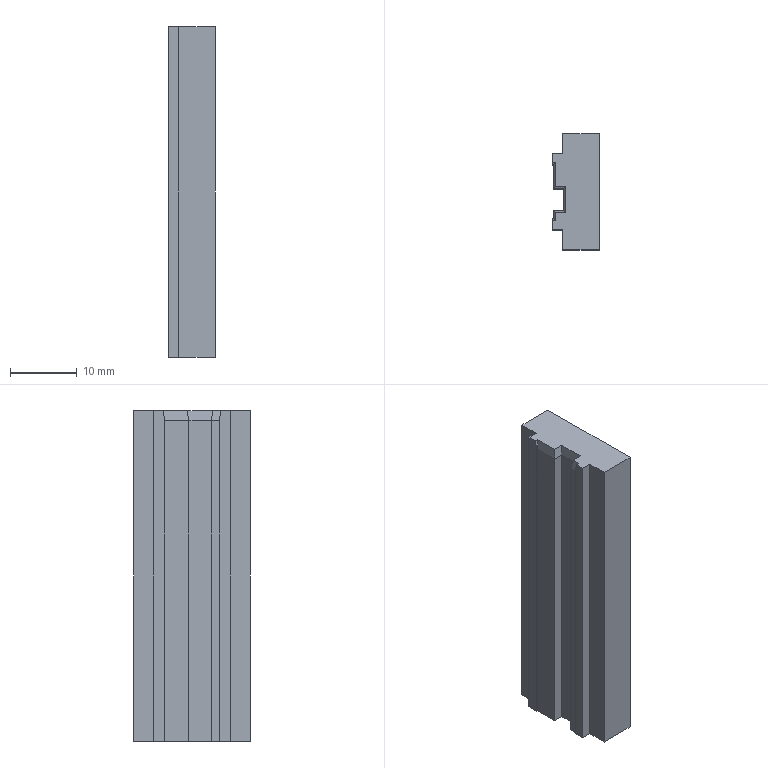Part | SolidWorks | features ICE 3, Chamfer 2, RefAxis 2, Extrusion 1, MirrorPattern 1, RevCut 1 | 1 solid | 33 faces | box 7 x 17.4 x 49.4 mm | volume 5230 mm3 | plane 25 | cone 4 | sphere 4
STEP:
#1=CARTESIAN_POINT('',(5.617,0.,19.076));
#2=VERTEX_POINT('',#1);
#3=CARTESIAN_POINT('',(5.617,0.,20.924));
#4=VERTEX_POINT('',#3);
#5=CARTESIAN_POINT('',(5.617,0.,20.));
#6=DIRECTION('',(1.,0.,0.));
#7=DIRECTION('',(0.,0.,-1.));
#8=AXIS2_PLACEMENT_3D('',#5,#6,#7);
#9=CIRCLE('',#8,0.9239);
#10=EDGE_CURVE('',#2,#4,#9,.T.);
#11=ORIENTED_EDGE('',*,*,#10,.F.);
#12=CARTESIAN_POINT('',(7.,0.,18.503));
#13=VERTEX_POINT('',#12);
#14=CARTESIAN_POINT('',(7.,0.,18.503));
#15=DIRECTION('',(0.9239,0.,-0.3827));
#16=VECTOR('',#15,1000.);
#17=LINE('',#14,#16);
#18=EDGE_CURVE('',#2,#13,#17,.T.);
#19=ORIENTED_EDGE('',*,*,#18,.T.);
#20=CARTESIAN_POINT('',(7.,0.,21.497));
#21=VERTEX_POINT('',#20);
#22=CARTESIAN_POINT('',(7.,0.,20.));
#23=DIRECTION('',(1.,0.,0.));
#24=DIRECTION('',(0.,0.,-1.));
#25=AXIS2_PLACEMENT_3D('',#22,#23,#24);
#26=CIRCLE('',#25,1.497);
#27=EDGE_CURVE('',#13,#21,#26,.T.);
#28=ORIENTED_EDGE('',*,*,#27,.T.);
#29=CARTESIAN_POINT('',(7.,0.,21.497));
#30=DIRECTION('',(0.9239,0.,0.3827));
#31=VECTOR('',#30,1000.);
#32=LINE('',#29,#31);
#33=EDGE_CURVE('',#4,#21,#32,.T.);
#34=ORIENTED_EDGE('',*,*,#33,.F.);
#35=EDGE_LOOP('',(#11,#19,#28,#34));
#36=FACE_OUTER_BOUND('',#35,.T.);
#37=CARTESIAN_POINT('',(7.,0.,20.));
#38=DIRECTION('',(1.,0.,0.));
#39=DIRECTION('',(0.,0.,1.));
#40=AXIS2_PLACEMENT_3D('',#37,#38,#39);
#41=CONICAL_SURFACE('',#40,1.497,0.3927);
#42=ADVANCED_FACE('',(#36),#41,.F.);
#43=CARTESIAN_POINT('',(5.617,0.,20.));
#44=DIRECTION('',(1.,0.,0.));
#45=DIRECTION('',(0.,0.,-1.));
#46=AXIS2_PLACEMENT_3D('',#43,#44,#45);
#47=CIRCLE('',#46,0.9239);
#48=EDGE_CURVE('',#4,#2,#47,.T.);
#49=ORIENTED_EDGE('',*,*,#48,.T.);
#50=CARTESIAN_POINT('',(5.,0.,20.));
#51=VERTEX_POINT('',#50);
#52=CARTESIAN_POINT('',(6.,0.,20.));
#53=DIRECTION('',(0.,1.,0.));
#54=DIRECTION('',(0.,0.,1.));
#55=AXIS2_PLACEMENT_3D('',#52,#53,#54);
#56=CIRCLE('',#55,1.);
#57=EDGE_CURVE('',#2,#51,#56,.T.);
#58=ORIENTED_EDGE('',*,*,#57,.T.);
#59=CARTESIAN_POINT('',(6.,0.,20.));
#60=DIRECTION('',(0.,-1.,0.));
#61=DIRECTION('',(0.,0.,-1.));
#62=AXIS2_PLACEMENT_3D('',#59,#60,#61);
#63=CIRCLE('',#62,1.);
#64=EDGE_CURVE('',#4,#51,#63,.T.);
#65=ORIENTED_EDGE('',*,*,#64,.F.);
#66=EDGE_LOOP('',(#49,#58,#65));
#67=FACE_OUTER_BOUND('',#66,.T.);
#68=CARTESIAN_POINT('',(6.,0.,20.));
#69=DIRECTION('',(0.,1.,0.));
#70=DIRECTION('',(0.,0.,1.));
#71=AXIS2_PLACEMENT_3D('',#68,#69,#70);
#72=SPHERICAL_SURFACE('',#71,1.);
#73=ADVANCED_FACE('',(#67),#72,.F.);
#74=CARTESIAN_POINT('',(5.617,0.,-20.924));
#75=VERTEX_POINT('',#74);
#76=CARTESIAN_POINT('',(5.617,0.,-19.076));
#77=VERTEX_POINT('',#76);
#78=CARTESIAN_POINT('',(5.617,0.,-20.));
#79=DIRECTION('',(-1.,0.,0.));
#80=DIRECTION('',(0.,0.,1.));
#81=AXIS2_PLACEMENT_3D('',#78,#79,#80);
#82=CIRCLE('',#81,0.9239);
#83=EDGE_CURVE('',#75,#77,#82,.T.);
#84=ORIENTED_EDGE('',*,*,#83,.T.);
#85=CARTESIAN_POINT('',(7.,0.,-18.503));
#86=VERTEX_POINT('',#85);
#87=CARTESIAN_POINT('',(7.,0.,-18.503));
#88=DIRECTION('',(0.9239,0.,0.3827));
#89=VECTOR('',#88,1000.);
#90=LINE('',#87,#89);
#91=EDGE_CURVE('',#77,#86,#90,.T.);
#92=ORIENTED_EDGE('',*,*,#91,.T.);
#93=CARTESIAN_POINT('',(7.,0.,-21.497));
#94=VERTEX_POINT('',#93);
#95=CARTESIAN_POINT('',(7.,0.,-20.));
#96=DIRECTION('',(-1.,0.,0.));
#97=DIRECTION('',(0.,0.,1.));
#98=AXIS2_PLACEMENT_3D('',#95,#96,#97);
#99=CIRCLE('',#98,1.497);
#100=EDGE_CURVE('',#94,#86,#99,.T.);
#101=ORIENTED_EDGE('',*,*,#100,.F.);
#102=CARTESIAN_POINT('',(7.,0.,-21.497));
#103=DIRECTION('',(0.9239,0.,-0.3827));
#104=VECTOR('',#103,1000.);
#105=LINE('',#102,#104);
#106=EDGE_CURVE('',#75,#94,#105,.T.);
#107=ORIENTED_EDGE('',*,*,#106,.F.);
#108=EDGE_LOOP('',(#84,#92,#101,#107));
#109=FACE_OUTER_BOUND('',#108,.T.);
#110=CARTESIAN_POINT('',(7.,0.,-20.));
#111=DIRECTION('',(1.,0.,0.));
#112=DIRECTION('',(0.,0.,-1.));
#113=AXIS2_PLACEMENT_3D('',#110,#111,#112);
#114=CONICAL_SURFACE('',#113,1.497,0.3927);
#115=ADVANCED_FACE('',(#109),#114,.F.);
#116=CARTESIAN_POINT('',(5.617,0.,-20.));
#117=DIRECTION('',(-1.,0.,0.));
#118=DIRECTION('',(0.,0.,1.));
#119=AXIS2_PLACEMENT_3D('',#116,#117,#118);
#120=CIRCLE('',#119,0.9239);
#121=EDGE_CURVE('',#77,#75,#120,.T.);
#122=ORIENTED_EDGE('',*,*,#121,.F.);
#123=CARTESIAN_POINT('',(5.,0.,-20.));
#124=VERTEX_POINT('',#123);
#125=CARTESIAN_POINT('',(6.,0.,-20.));
#126=DIRECTION('',(0.,-1.,0.));
#127=DIRECTION('',(0.,0.,-1.));
#128=AXIS2_PLACEMENT_3D('',#125,#126,#127);
#129=CIRCLE('',#128,1.);
#130=EDGE_CURVE('',#77,#124,#129,.T.);
#131=ORIENTED_EDGE('',*,*,#130,.T.);
#132=CARTESIAN_POINT('',(6.,0.,-20.));
#133=DIRECTION('',(0.,1.,0.));
#134=DIRECTION('',(0.,0.,1.));
#135=AXIS2_PLACEMENT_3D('',#132,#133,#134);
#136=CIRCLE('',#135,1.);
#137=EDGE_CURVE('',#75,#124,#136,.T.);
#138=ORIENTED_EDGE('',*,*,#137,.F.);
#139=EDGE_LOOP('',(#122,#131,#138));
#140=FACE_OUTER_BOUND('',#139,.T.);
#141=CARTESIAN_POINT('',(6.,0.,-20.));
#142=DIRECTION('',(0.,-1.,0.));
#143=DIRECTION('',(0.,0.,-1.));
#144=AXIS2_PLACEMENT_3D('',#141,#142,#143);
#145=SPHERICAL_SURFACE('',#144,1.);
#146=ADVANCED_FACE('',(#140),#145,.F.);
#147=CARTESIAN_POINT('',(1.5,8.7,24.7));
#148=VERTEX_POINT('',#147);
#149=CARTESIAN_POINT('',(1.5,8.7,-24.7));
#150=VERTEX_POINT('',#149);
#151=CARTESIAN_POINT('',(1.5,8.7,-24.7));
#152=DIRECTION('',(0.,0.,-1.));
#153=VECTOR('',#152,1000.);
#154=LINE('',#151,#153);
#155=EDGE_CURVE('',#148,#150,#154,.T.);
#156=ORIENTED_EDGE('',*,*,#155,.F.);
#157=CARTESIAN_POINT('',(7.,8.7,24.7));
#158=VERTEX_POINT('',#157);
#159=CARTESIAN_POINT('',(7.,8.7,24.7));
#160=DIRECTION('',(-1.,0.,0.));
#161=VECTOR('',#160,1000.);
#162=LINE('',#159,#161);
#163=EDGE_CURVE('',#158,#148,#162,.T.);
#164=ORIENTED_EDGE('',*,*,#163,.F.);
#165=CARTESIAN_POINT('',(7.,8.7,-24.7));
#166=VERTEX_POINT('',#165);
#167=CARTESIAN_POINT('',(7.,8.7,24.7));
#168=DIRECTION('',(0.,0.,1.));
#169=VECTOR('',#168,1000.);
#170=LINE('',#167,#169);
#171=EDGE_CURVE('',#166,#158,#170,.T.);
#172=ORIENTED_EDGE('',*,*,#171,.F.);
#173=CARTESIAN_POINT('',(7.,8.7,-24.7));
#174=DIRECTION('',(-1.,0.,0.));
#175=VECTOR('',#174,1000.);
#176=LINE('',#173,#175);
#177=EDGE_CURVE('',#166,#150,#176,.T.);
#178=ORIENTED_EDGE('',*,*,#177,.T.);
#179=EDGE_LOOP('',(#156,#164,#172,#178));
#180=FACE_OUTER_BOUND('',#179,.T.);
#181=CARTESIAN_POINT('',(7.,8.7,24.7));
#182=DIRECTION('',(0.,-1.,0.));
#183=DIRECTION('',(0.,0.,-1.));
#184=AXIS2_PLACEMENT_3D('',#181,#182,#183);
#185=PLANE('',#184);
#186=ADVANCED_FACE('',(#180),#185,.F.);
#187=ORIENTED_EDGE('',*,*,#100,.T.);
#188=CARTESIAN_POINT('',(7.,0.,-20.));
#189=DIRECTION('',(-1.,0.,0.));
#190=DIRECTION('',(0.,0.,1.));
#191=AXIS2_PLACEMENT_3D('',#188,#189,#190);
#192=CIRCLE('',#191,1.497);
#193=EDGE_CURVE('',#86,#94,#192,.T.);
#194=ORIENTED_EDGE('',*,*,#193,.T.);
#195=EDGE_LOOP('',(#187,#194));
#196=FACE_BOUND('',#195,.T.);
#197=CARTESIAN_POINT('',(7.,-8.7,-24.7));
#198=VERTEX_POINT('',#197);
#199=CARTESIAN_POINT('',(7.,8.7,-24.7));
#200=DIRECTION('',(0.,1.,0.));
#201=VECTOR('',#200,1000.);
#202=LINE('',#199,#201);
#203=EDGE_CURVE('',#198,#166,#202,.T.);
#204=ORIENTED_EDGE('',*,*,#203,.T.);
#205=ORIENTED_EDGE('',*,*,#171,.T.);
#206=CARTESIAN_POINT('',(7.,-8.7,24.7));
#207=VERTEX_POINT('',#206);
#208=CARTESIAN_POINT('',(7.,8.7,24.7));
#209=DIRECTION('',(0.,-1.,0.));
#210=VECTOR('',#209,1000.);
#211=LINE('',#208,#210);
#212=EDGE_CURVE('',#158,#207,#211,.T.);
#213=ORIENTED_EDGE('',*,*,#212,.T.);
#214=CARTESIAN_POINT('',(7.,-8.7,24.7));
#215=DIRECTION('',(0.,0.,-1.));
#216=VECTOR('',#215,1000.);
#217=LINE('',#214,#216);
#218=EDGE_CURVE('',#207,#198,#217,.T.);
#219=ORIENTED_EDGE('',*,*,#218,.T.);
#220=EDGE_LOOP('',(#204,#205,#213,#219));
#221=FACE_OUTER_BOUND('',#220,.T.);
#222=CARTESIAN_POINT('',(7.,0.,20.));
#223=DIRECTION('',(1.,0.,0.));
#224=DIRECTION('',(0.,0.,-1.));
#225=AXIS2_PLACEMENT_3D('',#222,#223,#224);
#226=CIRCLE('',#225,1.497);
#227=EDGE_CURVE('',#21,#13,#226,.T.);
#228=ORIENTED_EDGE('',*,*,#227,.F.);
#229=ORIENTED_EDGE('',*,*,#27,.F.);
#230=EDGE_LOOP('',(#228,#229));
#231=FACE_BOUND('',#230,.T.);
#232=CARTESIAN_POINT('',(7.,0.,0.));
#233=DIRECTION('',(1.,0.,0.));
#234=DIRECTION('',(0.,0.,-1.));
#235=AXIS2_PLACEMENT_3D('',#232,#233,#234);
#236=PLANE('',#235);
#237=ADVANCED_FACE('',(#196,#221,#231),#236,.T.);
#238=CARTESIAN_POINT('',(0.2,-4.05,-24.7));
#239=VERTEX_POINT('',#238);
#240=CARTESIAN_POINT('',(0.2,-4.05,23.2));
#241=VERTEX_POINT('',#240);
#242=CARTESIAN_POINT('',(0.2,-4.05,-24.7));
#243=DIRECTION('',(0.,0.,1.));
#244=VECTOR('',#243,1000.);
#245=LINE('',#242,#244);
#246=EDGE_CURVE('',#239,#241,#245,.T.);
#247=ORIENTED_EDGE('',*,*,#246,.T.);
#248=CARTESIAN_POINT('',(0.2,-2.85,23.2));
#249=VERTEX_POINT('',#248);
#250=CARTESIAN_POINT('',(0.2,-2.85,23.2));
#251=DIRECTION('',(0.,1.,0.));
#252=VECTOR('',#251,1000.);
#253=LINE('',#250,#252);
#254=EDGE_CURVE('',#241,#249,#253,.T.);
#255=ORIENTED_EDGE('',*,*,#254,.T.);
#256=CARTESIAN_POINT('',(0.2,-2.85,-24.7));
#257=VERTEX_POINT('',#256);
#258=CARTESIAN_POINT('',(0.2,-2.85,0.));
#259=DIRECTION('',(0.,0.,1.));
#260=VECTOR('',#259,1000.);
#261=LINE('',#258,#260);
#262=EDGE_CURVE('',#257,#249,#261,.T.);
#263=ORIENTED_EDGE('',*,*,#262,.F.);
#264=CARTESIAN_POINT('',(0.2,4.05,-24.7));
#265=DIRECTION('',(0.,-1.,0.));
#266=VECTOR('',#265,1000.);
#267=LINE('',#264,#266);
#268=EDGE_CURVE('',#257,#239,#267,.T.);
#269=ORIENTED_EDGE('',*,*,#268,.T.);
#270=EDGE_LOOP('',(#247,#255,#263,#269));
#271=FACE_OUTER_BOUND('',#270,.T.);
#272=CARTESIAN_POINT('',(0.2,0.,0.));
#273=DIRECTION('',(-1.,0.,0.));
#274=DIRECTION('',(0.,0.,1.));
#275=AXIS2_PLACEMENT_3D('',#272,#273,#274);
#276=PLANE('',#275);
#277=ADVANCED_FACE('',(#271),#276,.T.);
#278=CARTESIAN_POINT('',(0.,4.05,23.2));
#279=VERTEX_POINT('',#278);
#280=CARTESIAN_POINT('',(0.,4.05,-24.7));
#281=VERTEX_POINT('',#280);
#282=CARTESIAN_POINT('',(0.,4.05,-24.7));
#283=DIRECTION('',(0.,0.,-1.));
#284=VECTOR('',#283,1000.);
#285=LINE('',#282,#284);
#286=EDGE_CURVE('',#279,#281,#285,.T.);
#287=ORIENTED_EDGE('',*,*,#286,.F.);
#288=CARTESIAN_POINT('',(0.,4.35,24.7));
#289=VERTEX_POINT('',#288);
#290=CARTESIAN_POINT('',(0.,4.05,23.2));
#291=DIRECTION('',(0.,0.1961,0.9806));
#292=VECTOR('',#291,1000.);
#293=LINE('',#290,#292);
#294=EDGE_CURVE('',#279,#289,#293,.T.);
#295=ORIENTED_EDGE('',*,*,#294,.T.);
#296=CARTESIAN_POINT('',(0.,5.7,24.7));
#297=VERTEX_POINT('',#296);
#298=CARTESIAN_POINT('',(0.,8.7,24.7));
#299=DIRECTION('',(0.,-1.,0.));
#300=VECTOR('',#299,1000.);
#301=LINE('',#298,#300);
#302=EDGE_CURVE('',#297,#289,#301,.T.);
#303=ORIENTED_EDGE('',*,*,#302,.F.);
#304=CARTESIAN_POINT('',(0.,5.7,-24.7));
#305=VERTEX_POINT('',#304);
#306=CARTESIAN_POINT('',(0.,5.7,-24.7));
#307=DIRECTION('',(0.,0.,1.));
#308=VECTOR('',#307,1000.);
#309=LINE('',#306,#308);
#310=EDGE_CURVE('',#305,#297,#309,.T.);
#311=ORIENTED_EDGE('',*,*,#310,.F.);
#312=CARTESIAN_POINT('',(0.,8.7,-24.7));
#313=DIRECTION('',(0.,1.,0.));
#314=VECTOR('',#313,1000.);
#315=LINE('',#312,#314);
#316=EDGE_CURVE('',#281,#305,#315,.T.);
#317=ORIENTED_EDGE('',*,*,#316,.F.);
#318=EDGE_LOOP('',(#287,#295,#303,#311,#317));
#319=FACE_OUTER_BOUND('',#318,.T.);
#320=CARTESIAN_POINT('',(0.,0.,0.));
#321=DIRECTION('',(1.,0.,0.));
#322=DIRECTION('',(0.,0.,-1.));
#323=AXIS2_PLACEMENT_3D('',#320,#321,#322);
#324=PLANE('',#323);
#325=ADVANCED_FACE('',(#319),#324,.F.);
#326=ORIENTED_EDGE('',*,*,#316,.T.);
#327=CARTESIAN_POINT('',(1.5,5.7,-24.7));
#328=VERTEX_POINT('',#327);
#329=CARTESIAN_POINT('',(1.5,5.7,-24.7));
#330=DIRECTION('',(-1.,0.,0.));
#331=VECTOR('',#330,1000.);
#332=LINE('',#329,#331);
#333=EDGE_CURVE('',#328,#305,#332,.T.);
#334=ORIENTED_EDGE('',*,*,#333,.F.);
#335=CARTESIAN_POINT('',(1.5,8.7,-24.7));
#336=DIRECTION('',(0.,-1.,0.));
#337=VECTOR('',#336,1000.);
#338=LINE('',#335,#337);
#339=EDGE_CURVE('',#150,#328,#338,.T.);
#340=ORIENTED_EDGE('',*,*,#339,.F.);
#341=ORIENTED_EDGE('',*,*,#177,.F.);
#342=ORIENTED_EDGE('',*,*,#203,.F.);
#343=CARTESIAN_POINT('',(1.5,-8.7,-24.7));
#344=VERTEX_POINT('',#343);
#345=CARTESIAN_POINT('',(7.,-8.7,-24.7));
#346=DIRECTION('',(-1.,0.,0.));
#347=VECTOR('',#346,1000.);
#348=LINE('',#345,#347);
#349=EDGE_CURVE('',#198,#344,#348,.T.);
#350=ORIENTED_EDGE('',*,*,#349,.T.);
#351=CARTESIAN_POINT('',(1.5,-5.7,-24.7));
#352=VERTEX_POINT('',#351);
#353=CARTESIAN_POINT('',(1.5,-8.7,-24.7));
#354=DIRECTION('',(0.,-1.,0.));
#355=VECTOR('',#354,1000.);
#356=LINE('',#353,#355);
#357=EDGE_CURVE('',#352,#344,#356,.T.);
#358=ORIENTED_EDGE('',*,*,#357,.F.);
#359=CARTESIAN_POINT('',(0.,-5.7,-24.7));
#360=VERTEX_POINT('',#359);
#361=CARTESIAN_POINT('',(1.5,-5.7,-24.7));
#362=DIRECTION('',(-1.,0.,0.));
#363=VECTOR('',#362,1000.);
#364=LINE('',#361,#363);
#365=EDGE_CURVE('',#352,#360,#364,.T.);
#366=ORIENTED_EDGE('',*,*,#365,.T.);
#367=CARTESIAN_POINT('',(0.,-4.05,-24.7));
#368=VERTEX_POINT('',#367);
#369=CARTESIAN_POINT('',(0.,8.7,-24.7));
#370=DIRECTION('',(0.,1.,0.));
#371=VECTOR('',#370,1000.);
#372=LINE('',#369,#371);
#373=EDGE_CURVE('',#360,#368,#372,.T.);
#374=ORIENTED_EDGE('',*,*,#373,.T.);
#375=CARTESIAN_POINT('',(0.2,-4.05,-24.7));
#376=DIRECTION('',(-1.,0.,0.));
#377=VECTOR('',#376,1000.);
#378=LINE('',#375,#377);
#379=EDGE_CURVE('',#239,#368,#378,.T.);
#380=ORIENTED_EDGE('',*,*,#379,.F.);
#381=ORIENTED_EDGE('',*,*,#268,.F.);
#382=CARTESIAN_POINT('',(1.7,-2.85,-24.7));
#383=VERTEX_POINT('',#382);
#384=CARTESIAN_POINT('',(1.7,-2.85,-24.7));
#385=DIRECTION('',(-1.,0.,0.));
#386=VECTOR('',#385,1000.);
#387=LINE('',#384,#386);
#388=EDGE_CURVE('',#383,#257,#387,.T.);
#389=ORIENTED_EDGE('',*,*,#388,.F.);
#390=CARTESIAN_POINT('',(1.7,0.45,-24.7));
#391=VERTEX_POINT('',#390);
#392=CARTESIAN_POINT('',(1.7,-2.85,-24.7));
#393=DIRECTION('',(0.,-1.,0.));
#394=VECTOR('',#393,1000.);
#395=LINE('',#392,#394);
#396=EDGE_CURVE('',#391,#383,#395,.T.);
#397=ORIENTED_EDGE('',*,*,#396,.F.);
#398=CARTESIAN_POINT('',(0.2,0.45,-24.7));
#399=VERTEX_POINT('',#398);
#400=CARTESIAN_POINT('',(1.7,0.45,-24.7));
#401=DIRECTION('',(-1.,0.,0.));
#402=VECTOR('',#401,1000.);
#403=LINE('',#400,#402);
#404=EDGE_CURVE('',#391,#399,#403,.T.);
#405=ORIENTED_EDGE('',*,*,#404,.T.);
#406=CARTESIAN_POINT('',(0.2,4.05,-24.7));
#407=VERTEX_POINT('',#406);
#408=CARTESIAN_POINT('',(0.2,4.05,-24.7));
#409=DIRECTION('',(0.,-1.,0.));
#410=VECTOR('',#409,1000.);
#411=LINE('',#408,#410);
#412=EDGE_CURVE('',#407,#399,#411,.T.);
#413=ORIENTED_EDGE('',*,*,#412,.F.);
#414=CARTESIAN_POINT('',(0.2,4.05,-24.7));
#415=DIRECTION('',(-1.,0.,0.));
#416=VECTOR('',#415,1000.);
#417=LINE('',#414,#416);
#418=EDGE_CURVE('',#407,#281,#417,.T.);
#419=ORIENTED_EDGE('',*,*,#418,.T.);
#420=EDGE_LOOP('',(#326,#334,#340,#341,#342,#350,#358,#366,#374,#380,#381,#389,#397,#405,#413,#419));
#421=FACE_OUTER_BOUND('',#420,.T.);
#422=CARTESIAN_POINT('',(7.,8.7,-24.7));
#423=DIRECTION('',(0.,0.,1.));
#424=DIRECTION('',(1.,0.,0.));
#425=AXIS2_PLACEMENT_3D('',#422,#423,#424);
#426=PLANE('',#425);
#427=ADVANCED_FACE('',(#421),#426,.F.);
#428=CARTESIAN_POINT('',(2.,0.75,24.7));
#429=VERTEX_POINT('',#428);
#430=CARTESIAN_POINT('',(2.,-3.15,24.7));
#431=VERTEX_POINT('',#430);
#432=CARTESIAN_POINT('',(2.,-3.15,24.7));
#433=DIRECTION('',(0.,-1.,0.));
#434=VECTOR('',#433,1000.);
#435=LINE('',#432,#434);
#436=EDGE_CURVE('',#429,#431,#435,.T.);
#437=ORIENTED_EDGE('',*,*,#436,.T.);
#438=CARTESIAN_POINT('',(0.5,-3.15,24.7));
#439=VERTEX_POINT('',#438);
#440=CARTESIAN_POINT('',(7.,-3.15,24.7));
#441=DIRECTION('',(-1.,0.,0.));
#442=VECTOR('',#441,1000.);
#443=LINE('',#440,#442);
#444=EDGE_CURVE('',#431,#439,#443,.T.);
#445=ORIENTED_EDGE('',*,*,#444,.T.);
#446=CARTESIAN_POINT('',(0.5,-4.35,24.7));
#447=VERTEX_POINT('',#446);
#448=CARTESIAN_POINT('',(0.5,-4.05,24.7));
#449=DIRECTION('',(0.,-1.,0.));
#450=VECTOR('',#449,1000.);
#451=LINE('',#448,#450);
#452=EDGE_CURVE('',#439,#447,#451,.T.);
#453=ORIENTED_EDGE('',*,*,#452,.T.);
#454=CARTESIAN_POINT('',(0.,-4.35,24.7));
#455=VERTEX_POINT('',#454);
#456=CARTESIAN_POINT('',(7.,-4.35,24.7));
#457=DIRECTION('',(-1.,0.,0.));
#458=VECTOR('',#457,1000.);
#459=LINE('',#456,#458);
#460=EDGE_CURVE('',#447,#455,#459,.T.);
#461=ORIENTED_EDGE('',*,*,#460,.T.);
#462=CARTESIAN_POINT('',(0.,-5.7,24.7));
#463=VERTEX_POINT('',#462);
#464=CARTESIAN_POINT('',(0.,8.7,24.7));
#465=DIRECTION('',(0.,-1.,0.));
#466=VECTOR('',#465,1000.);
#467=LINE('',#464,#466);
#468=EDGE_CURVE('',#455,#463,#467,.T.);
#469=ORIENTED_EDGE('',*,*,#468,.T.);
#470=CARTESIAN_POINT('',(1.5,-5.7,24.7));
#471=VERTEX_POINT('',#470);
#472=CARTESIAN_POINT('',(1.5,-5.7,24.7));
#473=DIRECTION('',(-1.,0.,0.));
#474=VECTOR('',#473,1000.);
#475=LINE('',#472,#474);
#476=EDGE_CURVE('',#471,#463,#475,.T.);
#477=ORIENTED_EDGE('',*,*,#476,.F.);
#478=CARTESIAN_POINT('',(1.5,-8.7,24.7));
#479=VERTEX_POINT('',#478);
#480=CARTESIAN_POINT('',(1.5,-8.7,24.7));
#481=DIRECTION('',(0.,1.,0.));
#482=VECTOR('',#481,1000.);
#483=LINE('',#480,#482);
#484=EDGE_CURVE('',#479,#471,#483,.T.);
#485=ORIENTED_EDGE('',*,*,#484,.F.);
#486=CARTESIAN_POINT('',(7.,-8.7,24.7));
#487=DIRECTION('',(-1.,0.,0.));
#488=VECTOR('',#487,1000.);
#489=LINE('',#486,#488);
#490=EDGE_CURVE('',#207,#479,#489,.T.);
#491=ORIENTED_EDGE('',*,*,#490,.F.);
#492=ORIENTED_EDGE('',*,*,#212,.F.);
#493=ORIENTED_EDGE('',*,*,#163,.T.);
#494=CARTESIAN_POINT('',(1.5,5.7,24.7));
#495=VERTEX_POINT('',#494);
#496=CARTESIAN_POINT('',(1.5,8.7,24.7));
#497=DIRECTION('',(0.,1.,0.));
#498=VECTOR('',#497,1000.);
#499=LINE('',#496,#498);
#500=EDGE_CURVE('',#495,#148,#499,.T.);
#501=ORIENTED_EDGE('',*,*,#500,.F.);
#502=CARTESIAN_POINT('',(1.5,5.7,24.7));
#503=DIRECTION('',(-1.,0.,0.));
#504=VECTOR('',#503,1000.);
#505=LINE('',#502,#504);
#506=EDGE_CURVE('',#495,#297,#505,.T.);
#507=ORIENTED_EDGE('',*,*,#506,.T.);
#508=ORIENTED_EDGE('',*,*,#302,.T.);
#509=CARTESIAN_POINT('',(0.5,4.35,24.7));
#510=VERTEX_POINT('',#509);
#511=CARTESIAN_POINT('',(7.,4.35,24.7));
#512=DIRECTION('',(1.,0.,0.));
#513=VECTOR('',#512,1000.);
#514=LINE('',#511,#513);
#515=EDGE_CURVE('',#289,#510,#514,.T.);
#516=ORIENTED_EDGE('',*,*,#515,.T.);
#517=CARTESIAN_POINT('',(0.5,0.75,24.7));
#518=VERTEX_POINT('',#517);
#519=CARTESIAN_POINT('',(0.5,0.45,24.7));
#520=DIRECTION('',(0.,-1.,0.));
#521=VECTOR('',#520,1000.);
#522=LINE('',#519,#521);
#523=EDGE_CURVE('',#510,#518,#522,.T.);
#524=ORIENTED_EDGE('',*,*,#523,.T.);
#525=CARTESIAN_POINT('',(7.,0.75,24.7));
#526=DIRECTION('',(1.,0.,0.));
#527=VECTOR('',#526,1000.);
#528=LINE('',#525,#527);
#529=EDGE_CURVE('',#518,#429,#528,.T.);
#530=ORIENTED_EDGE('',*,*,#529,.T.);
#531=EDGE_LOOP('',(#437,#445,#453,#461,#469,#477,#485,#491,#492,#493,#501,#507,#508,#516,#524,#530));
#532=FACE_OUTER_BOUND('',#531,.T.);
#533=CARTESIAN_POINT('',(7.,8.7,24.7));
#534=DIRECTION('',(0.,0.,-1.));
#535=DIRECTION('',(0.,1.,0.));
#536=AXIS2_PLACEMENT_3D('',#533,#534,#535);
#537=PLANE('',#536);
#538=ADVANCED_FACE('',(#532),#537,.F.);
#539=ORIENTED_EDGE('',*,*,#490,.T.);
#540=CARTESIAN_POINT('',(1.5,-8.7,-24.7));
#541=DIRECTION('',(0.,0.,1.));
#542=VECTOR('',#541,1000.);
#543=LINE('',#540,#542);
#544=EDGE_CURVE('',#344,#479,#543,.T.);
#545=ORIENTED_EDGE('',*,*,#544,.F.);
#546=ORIENTED_EDGE('',*,*,#349,.F.);
#547=ORIENTED_EDGE('',*,*,#218,.F.);
#548=EDGE_LOOP('',(#539,#545,#546,#547));
#549=FACE_OUTER_BOUND('',#548,.T.);
#550=CARTESIAN_POINT('',(7.,-8.7,24.7));
#551=DIRECTION('',(0.,1.,0.));
#552=DIRECTION('',(0.,0.,1.));
#553=AXIS2_PLACEMENT_3D('',#550,#551,#552);
#554=PLANE('',#553);
#555=ADVANCED_FACE('',(#549),#554,.F.);
#556=ORIENTED_EDGE('',*,*,#468,.F.);
#557=CARTESIAN_POINT('',(0.,-4.05,23.2));
#558=VERTEX_POINT('',#557);
#559=CARTESIAN_POINT('',(0.,-4.35,24.7));
#560=DIRECTION('',(0.,0.1961,-0.9806));
#561=VECTOR('',#560,1000.);
#562=LINE('',#559,#561);
#563=EDGE_CURVE('',#455,#558,#562,.T.);
#564=ORIENTED_EDGE('',*,*,#563,.T.);
#565=CARTESIAN_POINT('',(0.,-4.05,-24.7));
#566=DIRECTION('',(0.,0.,1.));
#567=VECTOR('',#566,1000.);
#568=LINE('',#565,#567);
#569=EDGE_CURVE('',#368,#558,#568,.T.);
#570=ORIENTED_EDGE('',*,*,#569,.F.);
#571=ORIENTED_EDGE('',*,*,#373,.F.);
#572=CARTESIAN_POINT('',(0.,-5.7,-24.7));
#573=DIRECTION('',(0.,0.,-1.));
#574=VECTOR('',#573,1000.);
#575=LINE('',#572,#574);
#576=EDGE_CURVE('',#463,#360,#575,.T.);
#577=ORIENTED_EDGE('',*,*,#576,.F.);
#578=EDGE_LOOP('',(#556,#564,#570,#571,#577));
#579=FACE_OUTER_BOUND('',#578,.T.);
#580=CARTESIAN_POINT('',(0.,0.,0.));
#581=DIRECTION('',(1.,0.,0.));
#582=DIRECTION('',(0.,0.,-1.));
#583=AXIS2_PLACEMENT_3D('',#580,#581,#582);
#584=PLANE('',#583);
#585=ADVANCED_FACE('',(#579),#584,.F.);
#586=CARTESIAN_POINT('',(0.2,4.05,23.2));
#587=VERTEX_POINT('',#586);
#588=CARTESIAN_POINT('',(0.2,4.05,-24.7));
#589=DIRECTION('',(0.,0.,-1.));
#590=VECTOR('',#589,1000.);
#591=LINE('',#588,#590);
#592=EDGE_CURVE('',#587,#407,#591,.T.);
#593=ORIENTED_EDGE('',*,*,#592,.F.);
#594=CARTESIAN_POINT('',(0.2,4.05,23.2));
#595=DIRECTION('',(-1.,0.,0.));
#596=VECTOR('',#595,1000.);
#597=LINE('',#594,#596);
#598=EDGE_CURVE('',#587,#279,#597,.T.);
#599=ORIENTED_EDGE('',*,*,#598,.T.);
#600=ORIENTED_EDGE('',*,*,#286,.T.);
#601=ORIENTED_EDGE('',*,*,#418,.F.);
#602=EDGE_LOOP('',(#593,#599,#600,#601));
#603=FACE_OUTER_BOUND('',#602,.T.);
#604=CARTESIAN_POINT('',(0.2,4.05,-24.7));
#605=DIRECTION('',(0.,1.,0.));
#606=DIRECTION('',(0.,0.,1.));
#607=AXIS2_PLACEMENT_3D('',#604,#605,#606);
#608=PLANE('',#607);
#609=ADVANCED_FACE('',(#603),#608,.F.);
#610=ORIENTED_EDGE('',*,*,#569,.T.);
#611=CARTESIAN_POINT('',(0.2,-4.05,23.2));
#612=DIRECTION('',(1.,0.,0.));
#613=VECTOR('',#612,1000.);
#614=LINE('',#611,#613);
#615=EDGE_CURVE('',#558,#241,#614,.T.);
#616=ORIENTED_EDGE('',*,*,#615,.T.);
#617=ORIENTED_EDGE('',*,*,#246,.F.);
#618=ORIENTED_EDGE('',*,*,#379,.T.);
#619=EDGE_LOOP('',(#610,#616,#617,#618));
#620=FACE_OUTER_BOUND('',#619,.T.);
#621=CARTESIAN_POINT('',(0.2,-4.05,-24.7));
#622=DIRECTION('',(0.,-1.,0.));
#623=DIRECTION('',(0.,0.,-1.));
#624=AXIS2_PLACEMENT_3D('',#621,#622,#623);
#625=PLANE('',#624);
#626=ADVANCED_FACE('',(#620),#625,.F.);
#627=CARTESIAN_POINT('',(0.2,0.45,23.2));
#628=VERTEX_POINT('',#627);
#629=CARTESIAN_POINT('',(0.2,0.45,0.));
#630=DIRECTION('',(0.,0.,-1.));
#631=VECTOR('',#630,1000.);
#632=LINE('',#629,#631);
#633=EDGE_CURVE('',#628,#399,#632,.T.);
#634=ORIENTED_EDGE('',*,*,#633,.F.);
#635=CARTESIAN_POINT('',(0.2,4.05,23.2));
#636=DIRECTION('',(0.,1.,0.));
#637=VECTOR('',#636,1000.);
#638=LINE('',#635,#637);
#639=EDGE_CURVE('',#628,#587,#638,.T.);
#640=ORIENTED_EDGE('',*,*,#639,.T.);
#641=ORIENTED_EDGE('',*,*,#592,.T.);
#642=ORIENTED_EDGE('',*,*,#412,.T.);
#643=EDGE_LOOP('',(#634,#640,#641,#642));
#644=FACE_OUTER_BOUND('',#643,.T.);
#645=CARTESIAN_POINT('',(0.2,0.,0.));
#646=DIRECTION('',(-1.,0.,0.));
#647=DIRECTION('',(0.,0.,1.));
#648=AXIS2_PLACEMENT_3D('',#645,#646,#647);
#649=PLANE('',#648);
#650=ADVANCED_FACE('',(#644),#649,.T.);
#651=ORIENTED_EDGE('',*,*,#262,.T.);
#652=CARTESIAN_POINT('',(1.7,-2.85,23.2));
#653=VERTEX_POINT('',#652);
#654=CARTESIAN_POINT('',(1.7,-2.85,23.2));
#655=DIRECTION('',(1.,0.,0.));
#656=VECTOR('',#655,1000.);
#657=LINE('',#654,#656);
#658=EDGE_CURVE('',#249,#653,#657,.T.);
#659=ORIENTED_EDGE('',*,*,#658,.T.);
#660=CARTESIAN_POINT('',(1.7,-2.85,24.7));
#661=DIRECTION('',(0.,0.,1.));
#662=VECTOR('',#661,1000.);
#663=LINE('',#660,#662);
#664=EDGE_CURVE('',#383,#653,#663,.T.);
#665=ORIENTED_EDGE('',*,*,#664,.F.);
#666=ORIENTED_EDGE('',*,*,#388,.T.);
#667=EDGE_LOOP('',(#651,#659,#665,#666));
#668=FACE_OUTER_BOUND('',#667,.T.);
#669=CARTESIAN_POINT('',(1.7,-2.85,24.7));
#670=DIRECTION('',(0.,-1.,0.));
#671=DIRECTION('',(0.,0.,-1.));
#672=AXIS2_PLACEMENT_3D('',#669,#670,#671);
#673=PLANE('',#672);
#674=ADVANCED_FACE('',(#668),#673,.F.);
#675=CARTESIAN_POINT('',(1.7,0.45,23.2));
#676=VERTEX_POINT('',#675);
#677=CARTESIAN_POINT('',(1.7,0.45,24.7));
#678=DIRECTION('',(0.,0.,-1.));
#679=VECTOR('',#678,1000.);
#680=LINE('',#677,#679);
#681=EDGE_CURVE('',#676,#391,#680,.T.);
#682=ORIENTED_EDGE('',*,*,#681,.F.);
#683=CARTESIAN_POINT('',(1.7,0.45,23.2));
#684=DIRECTION('',(-1.,0.,0.));
#685=VECTOR('',#684,1000.);
#686=LINE('',#683,#685);
#687=EDGE_CURVE('',#676,#628,#686,.T.);
#688=ORIENTED_EDGE('',*,*,#687,.T.);
#689=ORIENTED_EDGE('',*,*,#633,.T.);
#690=ORIENTED_EDGE('',*,*,#404,.F.);
#691=EDGE_LOOP('',(#682,#688,#689,#690));
#692=FACE_OUTER_BOUND('',#691,.T.);
#693=CARTESIAN_POINT('',(1.7,0.45,24.7));
#694=DIRECTION('',(0.,1.,0.));
#695=DIRECTION('',(0.,0.,1.));
#696=AXIS2_PLACEMENT_3D('',#693,#694,#695);
#697=PLANE('',#696);
#698=ADVANCED_FACE('',(#692),#697,.F.);
#699=ORIENTED_EDGE('',*,*,#664,.T.);
#700=CARTESIAN_POINT('',(1.7,0.45,23.2));
#701=DIRECTION('',(0.,1.,0.));
#702=VECTOR('',#701,1000.);
#703=LINE('',#700,#702);
#704=EDGE_CURVE('',#653,#676,#703,.T.);
#705=ORIENTED_EDGE('',*,*,#704,.T.);
#706=ORIENTED_EDGE('',*,*,#681,.T.);
#707=ORIENTED_EDGE('',*,*,#396,.T.);
#708=EDGE_LOOP('',(#699,#705,#706,#707));
#709=FACE_OUTER_BOUND('',#708,.T.);
#710=CARTESIAN_POINT('',(1.7,0.,0.));
#711=DIRECTION('',(-1.,0.,0.));
#712=DIRECTION('',(0.,0.,1.));
#713=AXIS2_PLACEMENT_3D('',#710,#711,#712);
#714=PLANE('',#713);
#715=ADVANCED_FACE('',(#709),#714,.T.);
#716=ORIENTED_EDGE('',*,*,#130,.F.);
#717=ORIENTED_EDGE('',*,*,#83,.F.);
#718=ORIENTED_EDGE('',*,*,#137,.T.);
#719=EDGE_LOOP('',(#716,#717,#718));
#720=FACE_OUTER_BOUND('',#719,.T.);
#721=CARTESIAN_POINT('',(6.,0.,-20.));
#722=DIRECTION('',(0.,-1.,0.));
#723=DIRECTION('',(0.,0.,-1.));
#724=AXIS2_PLACEMENT_3D('',#721,#722,#723);
#725=SPHERICAL_SURFACE('',#724,1.);
#726=ADVANCED_FACE('',(#720),#725,.F.);
#727=ORIENTED_EDGE('',*,*,#91,.F.);
#728=ORIENTED_EDGE('',*,*,#121,.T.);
#729=ORIENTED_EDGE('',*,*,#106,.T.);
#730=ORIENTED_EDGE('',*,*,#193,.F.);
#731=EDGE_LOOP('',(#727,#728,#729,#730));
#732=FACE_OUTER_BOUND('',#731,.T.);
#733=CARTESIAN_POINT('',(7.,0.,-20.));
#734=DIRECTION('',(1.,0.,0.));
#735=DIRECTION('',(0.,0.,-1.));
#736=AXIS2_PLACEMENT_3D('',#733,#734,#735);
#737=CONICAL_SURFACE('',#736,1.497,0.3927);
#738=ADVANCED_FACE('',(#732),#737,.F.);
#739=ORIENTED_EDGE('',*,*,#57,.F.);
#740=ORIENTED_EDGE('',*,*,#10,.T.);
#741=ORIENTED_EDGE('',*,*,#64,.T.);
#742=EDGE_LOOP('',(#739,#740,#741));
#743=FACE_OUTER_BOUND('',#742,.T.);
#744=CARTESIAN_POINT('',(6.,0.,20.));
#745=DIRECTION('',(0.,1.,0.));
#746=DIRECTION('',(0.,0.,1.));
#747=AXIS2_PLACEMENT_3D('',#744,#745,#746);
#748=SPHERICAL_SURFACE('',#747,1.);
#749=ADVANCED_FACE('',(#743),#748,.F.);
#750=ORIENTED_EDGE('',*,*,#18,.F.);
#751=ORIENTED_EDGE('',*,*,#48,.F.);
#752=ORIENTED_EDGE('',*,*,#33,.T.);
#753=ORIENTED_EDGE('',*,*,#227,.T.);
#754=EDGE_LOOP('',(#750,#751,#752,#753));
#755=FACE_OUTER_BOUND('',#754,.T.);
#756=CARTESIAN_POINT('',(7.,0.,20.));
#757=DIRECTION('',(1.,0.,0.));
#758=DIRECTION('',(0.,0.,1.));
#759=AXIS2_PLACEMENT_3D('',#756,#757,#758);
#760=CONICAL_SURFACE('',#759,1.497,0.3927);
#761=ADVANCED_FACE('',(#755),#760,.F.);
#762=ORIENTED_EDGE('',*,*,#576,.T.);
#763=ORIENTED_EDGE('',*,*,#365,.F.);
#764=CARTESIAN_POINT('',(1.5,-5.7,-24.7));
#765=DIRECTION('',(0.,0.,-1.));
#766=VECTOR('',#765,1000.);
#767=LINE('',#764,#766);
#768=EDGE_CURVE('',#471,#352,#767,.T.);
#769=ORIENTED_EDGE('',*,*,#768,.F.);
#770=ORIENTED_EDGE('',*,*,#476,.T.);
#771=EDGE_LOOP('',(#762,#763,#769,#770));
#772=FACE_OUTER_BOUND('',#771,.T.);
#773=CARTESIAN_POINT('',(1.5,-5.7,-24.7));
#774=DIRECTION('',(0.,1.,0.));
#775=DIRECTION('',(0.,0.,1.));
#776=AXIS2_PLACEMENT_3D('',#773,#774,#775);
#777=PLANE('',#776);
#778=ADVANCED_FACE('',(#772),#777,.F.);
#779=ORIENTED_EDGE('',*,*,#357,.T.);
#780=ORIENTED_EDGE('',*,*,#544,.T.);
#781=ORIENTED_EDGE('',*,*,#484,.T.);
#782=ORIENTED_EDGE('',*,*,#768,.T.);
#783=EDGE_LOOP('',(#779,#780,#781,#782));
#784=FACE_OUTER_BOUND('',#783,.T.);
#785=CARTESIAN_POINT('',(1.5,0.,0.));
#786=DIRECTION('',(1.,0.,0.));
#787=DIRECTION('',(0.,0.,-1.));
#788=AXIS2_PLACEMENT_3D('',#785,#786,#787);
#789=PLANE('',#788);
#790=ADVANCED_FACE('',(#784),#789,.F.);
#791=ORIENTED_EDGE('',*,*,#310,.T.);
#792=ORIENTED_EDGE('',*,*,#506,.F.);
#793=CARTESIAN_POINT('',(1.5,5.7,-24.7));
#794=DIRECTION('',(0.,0.,1.));
#795=VECTOR('',#794,1000.);
#796=LINE('',#793,#795);
#797=EDGE_CURVE('',#328,#495,#796,.T.);
#798=ORIENTED_EDGE('',*,*,#797,.F.);
#799=ORIENTED_EDGE('',*,*,#333,.T.);
#800=EDGE_LOOP('',(#791,#792,#798,#799));
#801=FACE_OUTER_BOUND('',#800,.T.);
#802=CARTESIAN_POINT('',(1.5,5.7,-24.7));
#803=DIRECTION('',(0.,-1.,0.));
#804=DIRECTION('',(0.,0.,-1.));
#805=AXIS2_PLACEMENT_3D('',#802,#803,#804);
#806=PLANE('',#805);
#807=ADVANCED_FACE('',(#801),#806,.F.);
#808=ORIENTED_EDGE('',*,*,#339,.T.);
#809=ORIENTED_EDGE('',*,*,#797,.T.);
#810=ORIENTED_EDGE('',*,*,#500,.T.);
#811=ORIENTED_EDGE('',*,*,#155,.T.);
#812=EDGE_LOOP('',(#808,#809,#810,#811));
#813=FACE_OUTER_BOUND('',#812,.T.);
#814=CARTESIAN_POINT('',(1.5,0.,0.));
#815=DIRECTION('',(-1.,0.,0.));
#816=DIRECTION('',(0.,0.,1.));
#817=AXIS2_PLACEMENT_3D('',#814,#815,#816);
#818=PLANE('',#817);
#819=ADVANCED_FACE('',(#813),#818,.T.);
#820=ORIENTED_EDGE('',*,*,#563,.F.);
#821=ORIENTED_EDGE('',*,*,#460,.F.);
#822=CARTESIAN_POINT('',(0.05,-3.9,22.45));
#823=DIRECTION('',(0.1925,-0.1925,0.9623));
#824=VECTOR('',#823,1000.);
#825=LINE('',#822,#824);
#826=EDGE_CURVE('',#241,#447,#825,.T.);
#827=ORIENTED_EDGE('',*,*,#826,.F.);
#828=ORIENTED_EDGE('',*,*,#615,.F.);
#829=EDGE_LOOP('',(#820,#821,#827,#828));
#830=FACE_OUTER_BOUND('',#829,.T.);
#831=CARTESIAN_POINT('',(7.,-4.35,24.7));
#832=DIRECTION('',(0.,-0.9806,-0.1961));
#833=DIRECTION('',(-1.,0.,0.));
#834=AXIS2_PLACEMENT_3D('',#831,#832,#833);
#835=PLANE('',#834);
#836=ADVANCED_FACE('',(#830),#835,.F.);
#837=ORIENTED_EDGE('',*,*,#826,.T.);
#838=ORIENTED_EDGE('',*,*,#452,.F.);
#839=CARTESIAN_POINT('',(0.09444,-2.744,22.672));
#840=DIRECTION('',(0.1925,-0.1925,0.9623));
#841=VECTOR('',#840,1000.);
#842=LINE('',#839,#841);
#843=EDGE_CURVE('',#249,#439,#842,.T.);
#844=ORIENTED_EDGE('',*,*,#843,.F.);
#845=ORIENTED_EDGE('',*,*,#254,.F.);
#846=EDGE_LOOP('',(#837,#838,#844,#845));
#847=FACE_OUTER_BOUND('',#846,.T.);
#848=CARTESIAN_POINT('',(0.2,0.,23.2));
#849=DIRECTION('',(-0.9806,0.,0.1961));
#850=DIRECTION('',(0.,-1.,0.));
#851=AXIS2_PLACEMENT_3D('',#848,#849,#850);
#852=PLANE('',#851);
#853=ADVANCED_FACE('',(#847),#852,.T.);
#854=ORIENTED_EDGE('',*,*,#444,.F.);
#855=CARTESIAN_POINT('',(1.594,-2.744,22.672));
#856=DIRECTION('',(-0.1925,0.1925,-0.9623));
#857=VECTOR('',#856,1000.);
#858=LINE('',#855,#857);
#859=EDGE_CURVE('',#431,#653,#858,.T.);
#860=ORIENTED_EDGE('',*,*,#859,.T.);
#861=ORIENTED_EDGE('',*,*,#658,.F.);
#862=ORIENTED_EDGE('',*,*,#843,.T.);
#863=EDGE_LOOP('',(#854,#860,#861,#862));
#864=FACE_OUTER_BOUND('',#863,.T.);
#865=CARTESIAN_POINT('',(7.,-3.15,24.7));
#866=DIRECTION('',(0.,-0.9806,-0.1961));
#867=DIRECTION('',(-1.,0.,0.));
#868=AXIS2_PLACEMENT_3D('',#865,#866,#867);
#869=PLANE('',#868);
#870=ADVANCED_FACE('',(#864),#869,.F.);
#871=ORIENTED_EDGE('',*,*,#294,.F.);
#872=ORIENTED_EDGE('',*,*,#598,.F.);
#873=CARTESIAN_POINT('',(0.2,4.05,23.2));
#874=DIRECTION('',(-0.1925,-0.1925,-0.9623));
#875=VECTOR('',#874,1000.);
#876=LINE('',#873,#875);
#877=EDGE_CURVE('',#510,#587,#876,.T.);
#878=ORIENTED_EDGE('',*,*,#877,.F.);
#879=ORIENTED_EDGE('',*,*,#515,.F.);
#880=EDGE_LOOP('',(#871,#872,#878,#879));
#881=FACE_OUTER_BOUND('',#880,.T.);
#882=CARTESIAN_POINT('',(0.2,4.05,23.2));
#883=DIRECTION('',(0.,0.9806,-0.1961));
#884=DIRECTION('',(-1.,0.,0.));
#885=AXIS2_PLACEMENT_3D('',#882,#883,#884);
#886=PLANE('',#885);
#887=ADVANCED_FACE('',(#881),#886,.F.);
#888=ORIENTED_EDGE('',*,*,#877,.T.);
#889=ORIENTED_EDGE('',*,*,#639,.F.);
#890=CARTESIAN_POINT('',(0.2556,0.5056,23.478));
#891=DIRECTION('',(-0.1925,-0.1925,-0.9623));
#892=VECTOR('',#891,1000.);
#893=LINE('',#890,#892);
#894=EDGE_CURVE('',#518,#628,#893,.T.);
#895=ORIENTED_EDGE('',*,*,#894,.F.);
#896=ORIENTED_EDGE('',*,*,#523,.F.);
#897=EDGE_LOOP('',(#888,#889,#895,#896));
#898=FACE_OUTER_BOUND('',#897,.T.);
#899=CARTESIAN_POINT('',(0.2,0.,23.2));
#900=DIRECTION('',(-0.9806,0.,0.1961));
#901=DIRECTION('',(0.,-1.,0.));
#902=AXIS2_PLACEMENT_3D('',#899,#900,#901);
#903=PLANE('',#902);
#904=ADVANCED_FACE('',(#898),#903,.T.);
#905=ORIENTED_EDGE('',*,*,#894,.T.);
#906=ORIENTED_EDGE('',*,*,#687,.F.);
#907=CARTESIAN_POINT('',(1.683,0.4333,23.117));
#908=DIRECTION('',(-0.1925,-0.1925,-0.9623));
#909=VECTOR('',#908,1000.);
#910=LINE('',#907,#909);
#911=EDGE_CURVE('',#429,#676,#910,.T.);
#912=ORIENTED_EDGE('',*,*,#911,.F.);
#913=ORIENTED_EDGE('',*,*,#529,.F.);
#914=EDGE_LOOP('',(#905,#906,#912,#913));
#915=FACE_OUTER_BOUND('',#914,.T.);
#916=CARTESIAN_POINT('',(1.7,0.45,23.2));
#917=DIRECTION('',(0.,0.9806,-0.1961));
#918=DIRECTION('',(-1.,0.,0.));
#919=AXIS2_PLACEMENT_3D('',#916,#917,#918);
#920=PLANE('',#919);
#921=ADVANCED_FACE('',(#915),#920,.F.);
#922=ORIENTED_EDGE('',*,*,#859,.F.);
#923=ORIENTED_EDGE('',*,*,#436,.F.);
#924=ORIENTED_EDGE('',*,*,#911,.T.);
#925=ORIENTED_EDGE('',*,*,#704,.F.);
#926=EDGE_LOOP('',(#922,#923,#924,#925));
#927=FACE_OUTER_BOUND('',#926,.T.);
#928=CARTESIAN_POINT('',(1.7,0.,23.2));
#929=DIRECTION('',(-0.9806,0.,0.1961));
#930=DIRECTION('',(0.,-1.,0.));
#931=AXIS2_PLACEMENT_3D('',#928,#929,#930);
#932=PLANE('',#931);
#933=ADVANCED_FACE('',(#927),#932,.T.);
#934=CLOSED_SHELL('',(#42,#73,#115,#146,#186,#237,#277,#325,#427,#538,#555,#585,#609,#626,#650,#674,#698,#715,#726,#738,#749,#761,#778,#790,#807,#819,#836,#853,#870,#887,#904,#921,#933));
#935=MANIFOLD_SOLID_BREP('',#934);
#936=CARTESIAN_POINT('',(0.,0.,0.));
#937=DIRECTION('',(0.,0.,1.));
#938=DIRECTION('',(1.,0.,0.));
#939=AXIS2_PLACEMENT_3D('',#936,#937,#938);
#940=(LENGTH_UNIT()NAMED_UNIT(*)SI_UNIT(.MILLI.,.METRE.));
#941=UNCERTAINTY_MEASURE_WITH_UNIT(LENGTH_MEASURE(0.00001),#940,'','');
#942=(NAMED_UNIT(*)PLANE_ANGLE_UNIT()SI_UNIT($,.RADIAN.));
#943=(NAMED_UNIT(*)SI_UNIT($,.STERADIAN.)SOLID_ANGLE_UNIT());
#944=(GEOMETRIC_REPRESENTATION_CONTEXT(3)GLOBAL_UNCERTAINTY_ASSIGNED_CONTEXT((#941))GLOBAL_UNIT_ASSIGNED_CONTEXT((#940,#942,#943))REPRESENTATION_CONTEXT('',''));
#945=ADVANCED_BREP_SHAPE_REPRESENTATION('',(#935,#939),#944);